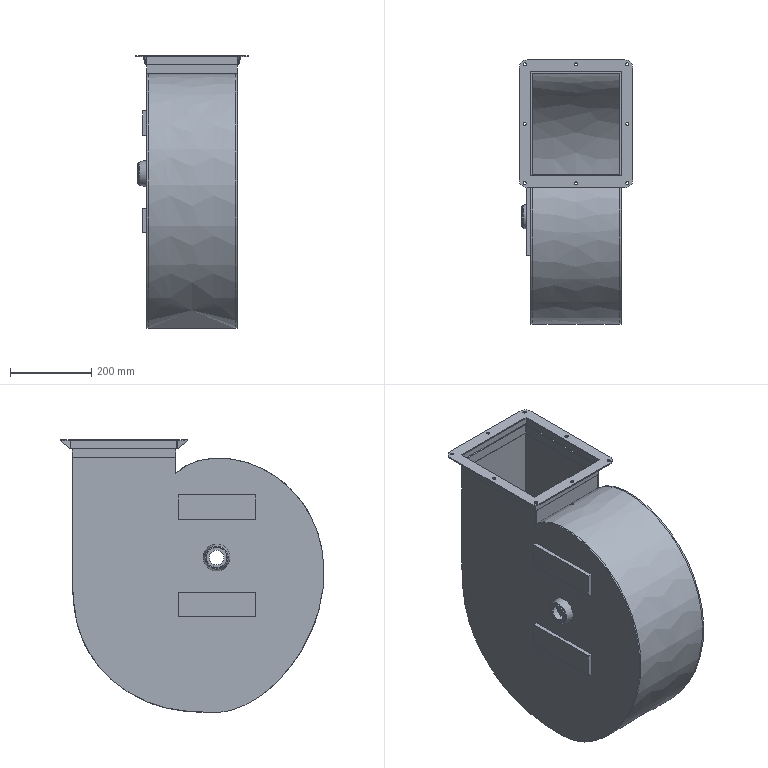Part | STEP file | wentylator 1V11 | 14 solids | 130 faces | box 280 x 648.901 x 670.864 mm | volume 4184150 mm3 | plane 82 | cylinder 32 | spline 16 | commonest cylinder face diameters 8 x20 40 x4 36 x2 50 x2 60 x2 200 x2